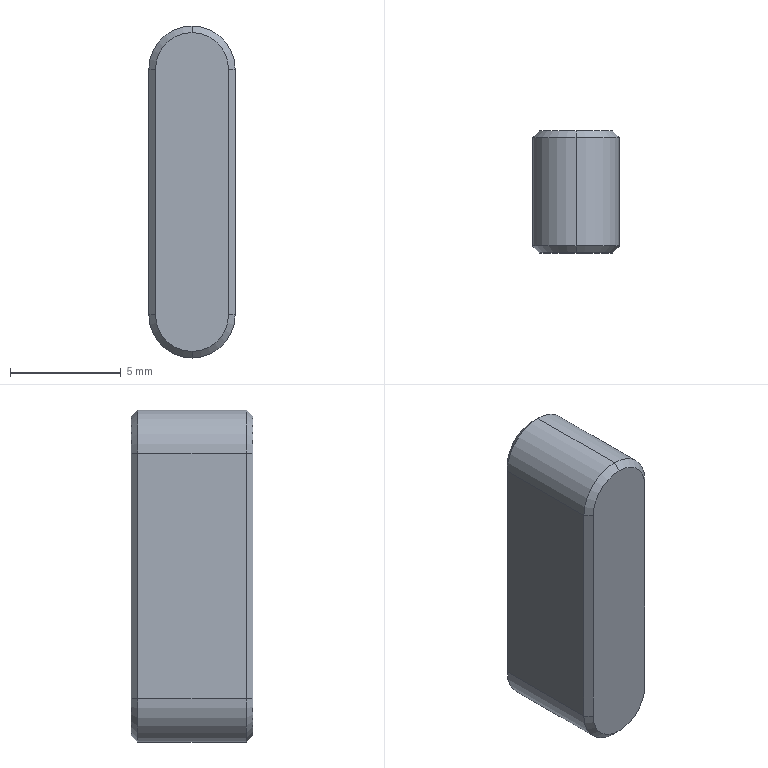Part | STEP file | Key 2 | 1 solid | 20 faces | box 3.9 x 5.5 x 15 mm | volume 300.753 mm3 | plane 8 | cone 8 | cylinder 4 | commonest cylinder face diameters 3.9 x4
STEP:
#1=CARTESIAN_POINT('',(0.,0.,0.));
#2=DIRECTION('',(0.,0.,1.));
#3=DIRECTION('',(1.,0.,0.));
#4=AXIS2_PLACEMENT_3D('',#1,#2,#3);
#5=CARTESIAN_POINT('',(1.95,2.45,13.05));
#6=VERTEX_POINT('',#5);
#7=CARTESIAN_POINT('',(1.95,-2.45,13.05));
#8=VERTEX_POINT('',#7);
#9=CARTESIAN_POINT('',(1.95,-2.75,13.05));
#10=DIRECTION('',(0.,-1.,0.));
#11=VECTOR('',#10,1.);
#12=LINE('',#9,#11);
#13=CARTESIAN_POINT('',(1.95,2.75,15.));
#14=DIRECTION('',(-1.,0.,0.));
#15=DIRECTION('',(0.,-1.,0.));
#16=AXIS2_PLACEMENT_3D('',#13,#14,#15);
#17=PLANE('',#16);
#18=CARTESIAN_POINT('',(5.5,-1.95));
#19=DIRECTION('',(1.,0.));
#20=VECTOR('',#19,1.);
#21=LINE('',#18,#20);
#22=(GEOMETRIC_REPRESENTATION_CONTEXT(2)PARAMETRIC_REPRESENTATION_CONTEXT()REPRESENTATION_CONTEXT('',''));
#23=DEFINITIONAL_REPRESENTATION('',(#21),#22);
#24=PCURVE('',#17,#23);
#25=CARTESIAN_POINT('',(0.,0.,13.05));
#26=DIRECTION('',(0.,-1.,0.));
#27=DIRECTION('',(1.,0.,0.));
#28=AXIS2_PLACEMENT_3D('',#25,#26,#27);
#29=CYLINDRICAL_SURFACE('',#28,1.95);
#30=CARTESIAN_POINT('',(0.,2.75));
#31=DIRECTION('',(0.,1.));
#32=VECTOR('',#31,1.);
#33=LINE('',#30,#32);
#34=(GEOMETRIC_REPRESENTATION_CONTEXT(2)PARAMETRIC_REPRESENTATION_CONTEXT()REPRESENTATION_CONTEXT('',''));
#35=DEFINITIONAL_REPRESENTATION('',(#33),#34);
#36=PCURVE('',#29,#35);
#37=SURFACE_CURVE('',#12,(#24,#36),.PCURVE_S1.);
#38=EDGE_CURVE('',#6,#8,#37,.T.);
#39=ORIENTED_EDGE('',*,*,#38,.T.);
#40=CARTESIAN_POINT('',(1.95,-2.45,1.95));
#41=VERTEX_POINT('',#40);
#42=CARTESIAN_POINT('',(1.95,-2.45,15.));
#43=DIRECTION('',(0.,0.,-1.));
#44=VECTOR('',#43,1.);
#45=LINE('',#42,#44);
#46=CARTESIAN_POINT('',(5.2,0.));
#47=DIRECTION('',(0.,-1.));
#48=VECTOR('',#47,1.);
#49=LINE('',#46,#48);
#50=(GEOMETRIC_REPRESENTATION_CONTEXT(2)PARAMETRIC_REPRESENTATION_CONTEXT()REPRESENTATION_CONTEXT('',''));
#51=DEFINITIONAL_REPRESENTATION('',(#49),#50);
#52=PCURVE('',#17,#51);
#53=CARTESIAN_POINT('',(1.95,-2.45,15.));
#54=DIRECTION('',(-0.7071,0.7071,0.));
#55=DIRECTION('',(0.,0.,-1.));
#56=AXIS2_PLACEMENT_3D('',#53,#54,#55);
#57=PLANE('',#56);
#58=CARTESIAN_POINT('',(0.,0.));
#59=DIRECTION('',(1.,0.));
#60=VECTOR('',#59,1.);
#61=LINE('',#58,#60);
#62=(GEOMETRIC_REPRESENTATION_CONTEXT(2)PARAMETRIC_REPRESENTATION_CONTEXT()REPRESENTATION_CONTEXT('',''));
#63=DEFINITIONAL_REPRESENTATION('',(#61),#62);
#64=PCURVE('',#57,#63);
#65=SURFACE_CURVE('',#45,(#52,#64),.PCURVE_S1.);
#66=EDGE_CURVE('',#8,#41,#65,.T.);
#67=ORIENTED_EDGE('',*,*,#66,.T.);
#68=CARTESIAN_POINT('',(1.95,2.45,1.95));
#69=VERTEX_POINT('',#68);
#70=CARTESIAN_POINT('',(1.95,2.75,1.95));
#71=DIRECTION('',(0.,1.,0.));
#72=VECTOR('',#71,1.);
#73=LINE('',#70,#72);
#74=CARTESIAN_POINT('',(0.,-13.05));
#75=DIRECTION('',(-1.,0.));
#76=VECTOR('',#75,1.);
#77=LINE('',#74,#76);
#78=(GEOMETRIC_REPRESENTATION_CONTEXT(2)PARAMETRIC_REPRESENTATION_CONTEXT()REPRESENTATION_CONTEXT('',''));
#79=DEFINITIONAL_REPRESENTATION('',(#77),#78);
#80=PCURVE('',#17,#79);
#81=CARTESIAN_POINT('',(0.,2.75,1.95));
#82=DIRECTION('',(0.,1.,0.));
#83=DIRECTION('',(-1.,0.,0.));
#84=AXIS2_PLACEMENT_3D('',#81,#82,#83);
#85=CYLINDRICAL_SURFACE('',#84,1.95);
#86=CARTESIAN_POINT('',(3.142,0.));
#87=DIRECTION('',(0.,1.));
#88=VECTOR('',#87,1.);
#89=LINE('',#86,#88);
#90=(GEOMETRIC_REPRESENTATION_CONTEXT(2)PARAMETRIC_REPRESENTATION_CONTEXT()REPRESENTATION_CONTEXT('',''));
#91=DEFINITIONAL_REPRESENTATION('',(#89),#90);
#92=PCURVE('',#85,#91);
#93=SURFACE_CURVE('',#73,(#80,#92),.PCURVE_S1.);
#94=EDGE_CURVE('',#41,#69,#93,.T.);
#95=ORIENTED_EDGE('',*,*,#94,.T.);
#96=CARTESIAN_POINT('',(1.95,2.45,15.));
#97=DIRECTION('',(0.,0.,1.));
#98=VECTOR('',#97,1.);
#99=LINE('',#96,#98);
#100=CARTESIAN_POINT('',(0.3,0.));
#101=DIRECTION('',(0.,1.));
#102=VECTOR('',#101,1.);
#103=LINE('',#100,#102);
#104=(GEOMETRIC_REPRESENTATION_CONTEXT(2)PARAMETRIC_REPRESENTATION_CONTEXT()REPRESENTATION_CONTEXT('',''));
#105=DEFINITIONAL_REPRESENTATION('',(#103),#104);
#106=PCURVE('',#17,#105);
#107=CARTESIAN_POINT('',(1.65,2.75,15.));
#108=DIRECTION('',(-0.7071,-0.7071,0.));
#109=DIRECTION('',(0.,0.,-1.));
#110=AXIS2_PLACEMENT_3D('',#107,#108,#109);
#111=PLANE('',#110);
#112=CARTESIAN_POINT('',(0.,0.4243));
#113=DIRECTION('',(-1.,0.));
#114=VECTOR('',#113,1.);
#115=LINE('',#112,#114);
#116=(GEOMETRIC_REPRESENTATION_CONTEXT(2)PARAMETRIC_REPRESENTATION_CONTEXT()REPRESENTATION_CONTEXT('',''));
#117=DEFINITIONAL_REPRESENTATION('',(#115),#116);
#118=PCURVE('',#111,#117);
#119=SURFACE_CURVE('',#99,(#106,#118),.PCURVE_S1.);
#120=EDGE_CURVE('',#69,#6,#119,.T.);
#121=ORIENTED_EDGE('',*,*,#120,.T.);
#122=EDGE_LOOP('',(#39,#67,#95,#121));
#123=FACE_BOUND('',#122,.T.);
#124=ADVANCED_FACE('',(#123),#17,.F.);
#125=CARTESIAN_POINT('',(0.,2.75,0.3));
#126=VERTEX_POINT('',#125);
#127=CARTESIAN_POINT('',(-1.65,2.75,1.95));
#128=VERTEX_POINT('',#127);
#129=CARTESIAN_POINT('',(0.,2.75,1.95));
#130=DIRECTION('',(0.,1.,0.));
#131=DIRECTION('',(0.,0.,-1.));
#132=AXIS2_PLACEMENT_3D('',#129,#130,#131);
#133=CIRCLE('',#132,1.65);
#134=CARTESIAN_POINT('',(-1.95,2.75,15.));
#135=DIRECTION('',(0.,-1.,0.));
#136=DIRECTION('',(0.,0.,-1.));
#137=AXIS2_PLACEMENT_3D('',#134,#135,#136);
#138=PLANE('',#137);
#139=CARTESIAN_POINT('',(14.7,1.95));
#140=CARTESIAN_POINT('',(14.7,-0.9079));
#141=CARTESIAN_POINT('',(12.225,0.5211));
#142=CARTESIAN_POINT('',(9.75,1.95));
#143=CARTESIAN_POINT('',(12.225,3.379));
#144=CARTESIAN_POINT('',(14.7,4.808));
#145=CARTESIAN_POINT('',(14.7,1.95));
#146=(BOUNDED_CURVE()B_SPLINE_CURVE(2,(#139,#140,#141,#142,#143,#144,#145),.UNSPECIFIED.,.T.,.F.)B_SPLINE_CURVE_WITH_KNOTS((1,2,2,2,2,1),(-2.094,0.,2.094,4.189,6.283,8.378),.UNSPECIFIED.)CURVE()GEOMETRIC_REPRESENTATION_ITEM()RATIONAL_B_SPLINE_CURVE((1.,0.5,1.,0.5,1.,0.5,1.))REPRESENTATION_ITEM(''));
#147=(GEOMETRIC_REPRESENTATION_CONTEXT(2)PARAMETRIC_REPRESENTATION_CONTEXT()REPRESENTATION_CONTEXT('',''));
#148=DEFINITIONAL_REPRESENTATION('',(#146),#147);
#149=PCURVE('',#138,#148);
#150=CARTESIAN_POINT('',(0.,2.75,1.95));
#151=DIRECTION('',(0.,-1.,0.));
#152=DIRECTION('',(1.,0.,0.));
#153=AXIS2_PLACEMENT_3D('',#150,#151,#152);
#154=CONICAL_SURFACE('',#153,1.65,0.7854);
#155=CARTESIAN_POINT('',(4.712,0.));
#156=DIRECTION('',(-1.,0.));
#157=VECTOR('',#156,1.);
#158=LINE('',#155,#157);
#159=(GEOMETRIC_REPRESENTATION_CONTEXT(2)PARAMETRIC_REPRESENTATION_CONTEXT()REPRESENTATION_CONTEXT('',''));
#160=DEFINITIONAL_REPRESENTATION('',(#158),#159);
#161=PCURVE('',#154,#160);
#162=SURFACE_CURVE('',#133,(#149,#161),.PCURVE_S1.);
#163=EDGE_CURVE('',#126,#128,#162,.T.);
#164=ORIENTED_EDGE('',*,*,#163,.T.);
#165=CARTESIAN_POINT('',(-1.65,2.75,13.05));
#166=VERTEX_POINT('',#165);
#167=CARTESIAN_POINT('',(-1.65,2.75,15.));
#168=DIRECTION('',(0.,0.,1.));
#169=VECTOR('',#168,1.);
#170=LINE('',#167,#169);
#171=CARTESIAN_POINT('',(0.,0.3));
#172=DIRECTION('',(-1.,0.));
#173=VECTOR('',#172,1.);
#174=LINE('',#171,#173);
#175=(GEOMETRIC_REPRESENTATION_CONTEXT(2)PARAMETRIC_REPRESENTATION_CONTEXT()REPRESENTATION_CONTEXT('',''));
#176=DEFINITIONAL_REPRESENTATION('',(#174),#175);
#177=PCURVE('',#138,#176);
#178=CARTESIAN_POINT('',(-1.95,2.45,15.));
#179=DIRECTION('',(0.7071,-0.7071,0.));
#180=DIRECTION('',(0.,0.,-1.));
#181=AXIS2_PLACEMENT_3D('',#178,#179,#180);
#182=PLANE('',#181);
#183=CARTESIAN_POINT('',(0.,0.4243));
#184=DIRECTION('',(-1.,0.));
#185=VECTOR('',#184,1.);
#186=LINE('',#183,#185);
#187=(GEOMETRIC_REPRESENTATION_CONTEXT(2)PARAMETRIC_REPRESENTATION_CONTEXT()REPRESENTATION_CONTEXT('',''));
#188=DEFINITIONAL_REPRESENTATION('',(#186),#187);
#189=PCURVE('',#182,#188);
#190=SURFACE_CURVE('',#170,(#177,#189),.PCURVE_S1.);
#191=EDGE_CURVE('',#128,#166,#190,.T.);
#192=ORIENTED_EDGE('',*,*,#191,.T.);
#193=CARTESIAN_POINT('',(0.,2.75,14.7));
#194=VERTEX_POINT('',#193);
#195=CARTESIAN_POINT('',(0.,2.75,13.05));
#196=DIRECTION('',(0.,1.,0.));
#197=DIRECTION('',(0.,0.,-1.));
#198=AXIS2_PLACEMENT_3D('',#195,#196,#197);
#199=CIRCLE('',#198,1.65);
#200=CARTESIAN_POINT('',(3.6,1.95));
#201=CARTESIAN_POINT('',(3.6,-0.9079));
#202=CARTESIAN_POINT('',(1.125,0.5211));
#203=CARTESIAN_POINT('',(-1.35,1.95));
#204=CARTESIAN_POINT('',(1.125,3.379));
#205=CARTESIAN_POINT('',(3.6,4.808));
#206=CARTESIAN_POINT('',(3.6,1.95));
#207=(BOUNDED_CURVE()B_SPLINE_CURVE(2,(#200,#201,#202,#203,#204,#205,#206),.UNSPECIFIED.,.T.,.F.)B_SPLINE_CURVE_WITH_KNOTS((1,2,2,2,2,1),(-2.094,0.,2.094,4.189,6.283,8.378),.UNSPECIFIED.)CURVE()GEOMETRIC_REPRESENTATION_ITEM()RATIONAL_B_SPLINE_CURVE((1.,0.5,1.,0.5,1.,0.5,1.))REPRESENTATION_ITEM(''));
#208=(GEOMETRIC_REPRESENTATION_CONTEXT(2)PARAMETRIC_REPRESENTATION_CONTEXT()REPRESENTATION_CONTEXT('',''));
#209=DEFINITIONAL_REPRESENTATION('',(#207),#208);
#210=PCURVE('',#138,#209);
#211=CARTESIAN_POINT('',(0.,2.75,13.05));
#212=DIRECTION('',(0.,-1.,0.));
#213=DIRECTION('',(1.,0.,0.));
#214=AXIS2_PLACEMENT_3D('',#211,#212,#213);
#215=CONICAL_SURFACE('',#214,1.65,0.7854);
#216=CARTESIAN_POINT('',(4.712,0.));
#217=DIRECTION('',(-1.,0.));
#218=VECTOR('',#217,1.);
#219=LINE('',#216,#218);
#220=(GEOMETRIC_REPRESENTATION_CONTEXT(2)PARAMETRIC_REPRESENTATION_CONTEXT()REPRESENTATION_CONTEXT('',''));
#221=DEFINITIONAL_REPRESENTATION('',(#219),#220);
#222=PCURVE('',#215,#221);
#223=SURFACE_CURVE('',#199,(#210,#222),.PCURVE_S1.);
#224=EDGE_CURVE('',#166,#194,#223,.T.);
#225=ORIENTED_EDGE('',*,*,#224,.T.);
#226=CARTESIAN_POINT('',(1.65,2.75,13.05));
#227=VERTEX_POINT('',#226);
#228=CARTESIAN_POINT('',(0.,2.75,13.05));
#229=DIRECTION('',(0.,1.,0.));
#230=DIRECTION('',(0.,0.,-1.));
#231=AXIS2_PLACEMENT_3D('',#228,#229,#230);
#232=CIRCLE('',#231,1.65);
#233=CARTESIAN_POINT('',(3.6,1.95));
#234=CARTESIAN_POINT('',(3.6,-0.9079));
#235=CARTESIAN_POINT('',(1.125,0.5211));
#236=CARTESIAN_POINT('',(-1.35,1.95));
#237=CARTESIAN_POINT('',(1.125,3.379));
#238=CARTESIAN_POINT('',(3.6,4.808));
#239=CARTESIAN_POINT('',(3.6,1.95));
#240=(BOUNDED_CURVE()B_SPLINE_CURVE(2,(#233,#234,#235,#236,#237,#238,#239),.UNSPECIFIED.,.T.,.F.)B_SPLINE_CURVE_WITH_KNOTS((1,2,2,2,2,1),(-2.094,0.,2.094,4.189,6.283,8.378),.UNSPECIFIED.)CURVE()GEOMETRIC_REPRESENTATION_ITEM()RATIONAL_B_SPLINE_CURVE((1.,0.5,1.,0.5,1.,0.5,1.))REPRESENTATION_ITEM(''));
#241=(GEOMETRIC_REPRESENTATION_CONTEXT(2)PARAMETRIC_REPRESENTATION_CONTEXT()REPRESENTATION_CONTEXT('',''));
#242=DEFINITIONAL_REPRESENTATION('',(#240),#241);
#243=PCURVE('',#138,#242);
#244=CARTESIAN_POINT('',(0.,2.75,13.05));
#245=DIRECTION('',(0.,-1.,0.));
#246=DIRECTION('',(1.,0.,0.));
#247=AXIS2_PLACEMENT_3D('',#244,#245,#246);
#248=CONICAL_SURFACE('',#247,1.65,0.7854);
#249=CARTESIAN_POINT('',(4.712,0.));
#250=DIRECTION('',(-1.,0.));
#251=VECTOR('',#250,1.);
#252=LINE('',#249,#251);
#253=(GEOMETRIC_REPRESENTATION_CONTEXT(2)PARAMETRIC_REPRESENTATION_CONTEXT()REPRESENTATION_CONTEXT('',''));
#254=DEFINITIONAL_REPRESENTATION('',(#252),#253);
#255=PCURVE('',#248,#254);
#256=SURFACE_CURVE('',#232,(#243,#255),.PCURVE_S1.);
#257=EDGE_CURVE('',#194,#227,#256,.T.);
#258=ORIENTED_EDGE('',*,*,#257,.T.);
#259=CARTESIAN_POINT('',(1.65,2.75,1.95));
#260=VERTEX_POINT('',#259);
#261=CARTESIAN_POINT('',(1.65,2.75,15.));
#262=DIRECTION('',(0.,0.,-1.));
#263=VECTOR('',#262,1.);
#264=LINE('',#261,#263);
#265=CARTESIAN_POINT('',(0.,3.6));
#266=DIRECTION('',(1.,0.));
#267=VECTOR('',#266,1.);
#268=LINE('',#265,#267);
#269=(GEOMETRIC_REPRESENTATION_CONTEXT(2)PARAMETRIC_REPRESENTATION_CONTEXT()REPRESENTATION_CONTEXT('',''));
#270=DEFINITIONAL_REPRESENTATION('',(#268),#269);
#271=PCURVE('',#138,#270);
#272=CARTESIAN_POINT('',(0.,0.));
#273=DIRECTION('',(1.,0.));
#274=VECTOR('',#273,1.);
#275=LINE('',#272,#274);
#276=(GEOMETRIC_REPRESENTATION_CONTEXT(2)PARAMETRIC_REPRESENTATION_CONTEXT()REPRESENTATION_CONTEXT('',''));
#277=DEFINITIONAL_REPRESENTATION('',(#275),#276);
#278=PCURVE('',#111,#277);
#279=SURFACE_CURVE('',#264,(#271,#278),.PCURVE_S1.);
#280=EDGE_CURVE('',#227,#260,#279,.T.);
#281=ORIENTED_EDGE('',*,*,#280,.T.);
#282=CARTESIAN_POINT('',(0.,2.75,1.95));
#283=DIRECTION('',(0.,1.,0.));
#284=DIRECTION('',(0.,0.,-1.));
#285=AXIS2_PLACEMENT_3D('',#282,#283,#284);
#286=CIRCLE('',#285,1.65);
#287=CARTESIAN_POINT('',(14.7,1.95));
#288=CARTESIAN_POINT('',(14.7,-0.9079));
#289=CARTESIAN_POINT('',(12.225,0.5211));
#290=CARTESIAN_POINT('',(9.75,1.95));
#291=CARTESIAN_POINT('',(12.225,3.379));
#292=CARTESIAN_POINT('',(14.7,4.808));
#293=CARTESIAN_POINT('',(14.7,1.95));
#294=(BOUNDED_CURVE()B_SPLINE_CURVE(2,(#287,#288,#289,#290,#291,#292,#293),.UNSPECIFIED.,.T.,.F.)B_SPLINE_CURVE_WITH_KNOTS((1,2,2,2,2,1),(-2.094,0.,2.094,4.189,6.283,8.378),.UNSPECIFIED.)CURVE()GEOMETRIC_REPRESENTATION_ITEM()RATIONAL_B_SPLINE_CURVE((1.,0.5,1.,0.5,1.,0.5,1.))REPRESENTATION_ITEM(''));
#295=(GEOMETRIC_REPRESENTATION_CONTEXT(2)PARAMETRIC_REPRESENTATION_CONTEXT()REPRESENTATION_CONTEXT('',''));
#296=DEFINITIONAL_REPRESENTATION('',(#294),#295);
#297=PCURVE('',#138,#296);
#298=CARTESIAN_POINT('',(0.,2.75,1.95));
#299=DIRECTION('',(0.,-1.,0.));
#300=DIRECTION('',(1.,0.,0.));
#301=AXIS2_PLACEMENT_3D('',#298,#299,#300);
#302=CONICAL_SURFACE('',#301,1.65,0.7854);
#303=CARTESIAN_POINT('',(10.996,0.));
#304=DIRECTION('',(-1.,0.));
#305=VECTOR('',#304,1.);
#306=LINE('',#303,#305);
#307=(GEOMETRIC_REPRESENTATION_CONTEXT(2)PARAMETRIC_REPRESENTATION_CONTEXT()REPRESENTATION_CONTEXT('',''));
#308=DEFINITIONAL_REPRESENTATION('',(#306),#307);
#309=PCURVE('',#302,#308);
#310=SURFACE_CURVE('',#286,(#297,#309),.PCURVE_S1.);
#311=EDGE_CURVE('',#260,#126,#310,.T.);
#312=ORIENTED_EDGE('',*,*,#311,.T.);
#313=EDGE_LOOP('',(#164,#192,#225,#258,#281,#312));
#314=FACE_BOUND('',#313,.T.);
#315=ADVANCED_FACE('',(#314),#138,.F.);
#316=CARTESIAN_POINT('',(-1.95,2.45,1.95));
#317=VERTEX_POINT('',#316);
#318=CARTESIAN_POINT('',(-1.95,-2.45,1.95));
#319=VERTEX_POINT('',#318);
#320=CARTESIAN_POINT('',(-1.95,2.75,1.95));
#321=DIRECTION('',(0.,-1.,0.));
#322=VECTOR('',#321,1.);
#323=LINE('',#320,#322);
#324=CARTESIAN_POINT('',(-1.95,2.75,15.));
#325=DIRECTION('',(1.,0.,0.));
#326=DIRECTION('',(0.,1.,0.));
#327=AXIS2_PLACEMENT_3D('',#324,#325,#326);
#328=PLANE('',#327);
#329=CARTESIAN_POINT('',(0.,-13.05));
#330=DIRECTION('',(-1.,0.));
#331=VECTOR('',#330,1.);
#332=LINE('',#329,#331);
#333=(GEOMETRIC_REPRESENTATION_CONTEXT(2)PARAMETRIC_REPRESENTATION_CONTEXT()REPRESENTATION_CONTEXT('',''));
#334=DEFINITIONAL_REPRESENTATION('',(#332),#333);
#335=PCURVE('',#328,#334);
#336=CARTESIAN_POINT('',(0.,2.75,1.95));
#337=DIRECTION('',(0.,-1.,0.));
#338=DIRECTION('',(1.,0.,0.));
#339=AXIS2_PLACEMENT_3D('',#336,#337,#338);
#340=CYLINDRICAL_SURFACE('',#339,1.95);
#341=CARTESIAN_POINT('',(3.142,0.));
#342=DIRECTION('',(0.,1.));
#343=VECTOR('',#342,1.);
#344=LINE('',#341,#343);
#345=(GEOMETRIC_REPRESENTATION_CONTEXT(2)PARAMETRIC_REPRESENTATION_CONTEXT()REPRESENTATION_CONTEXT('',''));
#346=DEFINITIONAL_REPRESENTATION('',(#344),#345);
#347=PCURVE('',#340,#346);
#348=SURFACE_CURVE('',#323,(#335,#347),.PCURVE_S1.);
#349=EDGE_CURVE('',#317,#319,#348,.T.);
#350=ORIENTED_EDGE('',*,*,#349,.T.);
#351=CARTESIAN_POINT('',(-1.95,-2.45,13.05));
#352=VERTEX_POINT('',#351);
#353=CARTESIAN_POINT('',(-1.95,-2.45,15.));
#354=DIRECTION('',(0.,0.,1.));
#355=VECTOR('',#354,1.);
#356=LINE('',#353,#355);
#357=CARTESIAN_POINT('',(-5.2,0.));
#358=DIRECTION('',(0.,1.));
#359=VECTOR('',#358,1.);
#360=LINE('',#357,#359);
#361=(GEOMETRIC_REPRESENTATION_CONTEXT(2)PARAMETRIC_REPRESENTATION_CONTEXT()REPRESENTATION_CONTEXT('',''));
#362=DEFINITIONAL_REPRESENTATION('',(#360),#361);
#363=PCURVE('',#328,#362);
#364=CARTESIAN_POINT('',(-1.65,-2.75,15.));
#365=DIRECTION('',(0.7071,0.7071,0.));
#366=DIRECTION('',(0.,0.,-1.));
#367=AXIS2_PLACEMENT_3D('',#364,#365,#366);
#368=PLANE('',#367);
#369=CARTESIAN_POINT('',(0.,0.4243));
#370=DIRECTION('',(-1.,0.));
#371=VECTOR('',#370,1.);
#372=LINE('',#369,#371);
#373=(GEOMETRIC_REPRESENTATION_CONTEXT(2)PARAMETRIC_REPRESENTATION_CONTEXT()REPRESENTATION_CONTEXT('',''));
#374=DEFINITIONAL_REPRESENTATION('',(#372),#373);
#375=PCURVE('',#368,#374);
#376=SURFACE_CURVE('',#356,(#363,#375),.PCURVE_S1.);
#377=EDGE_CURVE('',#319,#352,#376,.T.);
#378=ORIENTED_EDGE('',*,*,#377,.T.);
#379=CARTESIAN_POINT('',(-1.95,2.45,13.05));
#380=VERTEX_POINT('',#379);
#381=CARTESIAN_POINT('',(-1.95,2.75,13.05));
#382=DIRECTION('',(0.,1.,0.));
#383=VECTOR('',#382,1.);
#384=LINE('',#381,#383);
#385=CARTESIAN_POINT('',(0.,-1.95));
#386=DIRECTION('',(1.,0.));
#387=VECTOR('',#386,1.);
#388=LINE('',#385,#387);
#389=(GEOMETRIC_REPRESENTATION_CONTEXT(2)PARAMETRIC_REPRESENTATION_CONTEXT()REPRESENTATION_CONTEXT('',''));
#390=DEFINITIONAL_REPRESENTATION('',(#388),#389);
#391=PCURVE('',#328,#390);
#392=CARTESIAN_POINT('',(0.,0.,13.05));
#393=DIRECTION('',(0.,1.,0.));
#394=DIRECTION('',(-1.,0.,0.));
#395=AXIS2_PLACEMENT_3D('',#392,#393,#394);
#396=CYLINDRICAL_SURFACE('',#395,1.95);
#397=CARTESIAN_POINT('',(0.,2.75));
#398=DIRECTION('',(0.,1.));
#399=VECTOR('',#398,1.);
#400=LINE('',#397,#399);
#401=(GEOMETRIC_REPRESENTATION_CONTEXT(2)PARAMETRIC_REPRESENTATION_CONTEXT()REPRESENTATION_CONTEXT('',''));
#402=DEFINITIONAL_REPRESENTATION('',(#400),#401);
#403=PCURVE('',#396,#402);
#404=SURFACE_CURVE('',#384,(#391,#403),.PCURVE_S1.);
#405=EDGE_CURVE('',#352,#380,#404,.T.);
#406=ORIENTED_EDGE('',*,*,#405,.T.);
#407=CARTESIAN_POINT('',(-1.95,2.45,15.));
#408=DIRECTION('',(0.,0.,-1.));
#409=VECTOR('',#408,1.);
#410=LINE('',#407,#409);
#411=CARTESIAN_POINT('',(-0.3,0.));
#412=DIRECTION('',(0.,-1.));
#413=VECTOR('',#412,1.);
#414=LINE('',#411,#413);
#415=(GEOMETRIC_REPRESENTATION_CONTEXT(2)PARAMETRIC_REPRESENTATION_CONTEXT()REPRESENTATION_CONTEXT('',''));
#416=DEFINITIONAL_REPRESENTATION('',(#414),#415);
#417=PCURVE('',#328,#416);
#418=CARTESIAN_POINT('',(0.,0.));
#419=DIRECTION('',(1.,0.));
#420=VECTOR('',#419,1.);
#421=LINE('',#418,#420);
#422=(GEOMETRIC_REPRESENTATION_CONTEXT(2)PARAMETRIC_REPRESENTATION_CONTEXT()REPRESENTATION_CONTEXT('',''));
#423=DEFINITIONAL_REPRESENTATION('',(#421),#422);
#424=PCURVE('',#182,#423);
#425=SURFACE_CURVE('',#410,(#417,#424),.PCURVE_S1.);
#426=EDGE_CURVE('',#380,#317,#425,.T.);
#427=ORIENTED_EDGE('',*,*,#426,.T.);
#428=EDGE_LOOP('',(#350,#378,#406,#427));
#429=FACE_BOUND('',#428,.T.);
#430=ADVANCED_FACE('',(#429),#328,.F.);
#431=CARTESIAN_POINT('',(0.,-2.75,14.7));
#432=VERTEX_POINT('',#431);
#433=CARTESIAN_POINT('',(-1.65,-2.75,13.05));
#434=VERTEX_POINT('',#433);
#435=CARTESIAN_POINT('',(0.,-2.75,13.05));
#436=DIRECTION('',(0.,-1.,0.));
#437=DIRECTION('',(0.,0.,1.));
#438=AXIS2_PLACEMENT_3D('',#435,#436,#437);
#439=CIRCLE('',#438,1.65);
#440=CARTESIAN_POINT('',(-1.95,-2.75,15.));
#441=DIRECTION('',(0.,1.,0.));
#442=DIRECTION('',(0.,0.,1.));
#443=AXIS2_PLACEMENT_3D('',#440,#441,#442);
#444=PLANE('',#443);
#445=CARTESIAN_POINT('',(-0.3,1.95));
#446=CARTESIAN_POINT('',(-0.3,-0.9079));
#447=CARTESIAN_POINT('',(-2.775,0.5211));
#448=CARTESIAN_POINT('',(-5.25,1.95));
#449=CARTESIAN_POINT('',(-2.775,3.379));
#450=CARTESIAN_POINT('',(-0.3,4.808));
#451=CARTESIAN_POINT('',(-0.3,1.95));
#452=(BOUNDED_CURVE()B_SPLINE_CURVE(2,(#445,#446,#447,#448,#449,#450,#451),.UNSPECIFIED.,.T.,.F.)B_SPLINE_CURVE_WITH_KNOTS((1,2,2,2,2,1),(-2.094,0.,2.094,4.189,6.283,8.378),.UNSPECIFIED.)CURVE()GEOMETRIC_REPRESENTATION_ITEM()RATIONAL_B_SPLINE_CURVE((1.,0.5,1.,0.5,1.,0.5,1.))REPRESENTATION_ITEM(''));
#453=(GEOMETRIC_REPRESENTATION_CONTEXT(2)PARAMETRIC_REPRESENTATION_CONTEXT()REPRESENTATION_CONTEXT('',''));
#454=DEFINITIONAL_REPRESENTATION('',(#452),#453);
#455=PCURVE('',#444,#454);
#456=CARTESIAN_POINT('',(0.,-2.75,13.05));
#457=DIRECTION('',(0.,1.,0.));
#458=DIRECTION('',(-1.,0.,0.));
#459=AXIS2_PLACEMENT_3D('',#456,#457,#458);
#460=CONICAL_SURFACE('',#459,1.65,0.7854);
#461=CARTESIAN_POINT('',(1.571,0.));
#462=DIRECTION('',(-1.,0.));
#463=VECTOR('',#462,1.);
#464=LINE('',#461,#463);
#465=(GEOMETRIC_REPRESENTATION_CONTEXT(2)PARAMETRIC_REPRESENTATION_CONTEXT()REPRESENTATION_CONTEXT('',''));
#466=DEFINITIONAL_REPRESENTATION('',(#464),#465);
#467=PCURVE('',#460,#466);
#468=SURFACE_CURVE('',#439,(#455,#467),.PCURVE_S1.);
#469=EDGE_CURVE('',#432,#434,#468,.T.);
#470=ORIENTED_EDGE('',*,*,#469,.T.);
#471=CARTESIAN_POINT('',(-1.65,-2.75,1.95));
#472=VERTEX_POINT('',#471);
#473=CARTESIAN_POINT('',(-1.65,-2.75,15.));
#474=DIRECTION('',(0.,0.,-1.));
#475=VECTOR('',#474,1.);
#476=LINE('',#473,#475);
#477=CARTESIAN_POINT('',(0.,0.3));
#478=DIRECTION('',(-1.,0.));
#479=VECTOR('',#478,1.);
#480=LINE('',#477,#479);
#481=(GEOMETRIC_REPRESENTATION_CONTEXT(2)PARAMETRIC_REPRESENTATION_CONTEXT()REPRESENTATION_CONTEXT('',''));
#482=DEFINITIONAL_REPRESENTATION('',(#480),#481);
#483=PCURVE('',#444,#482);
#484=CARTESIAN_POINT('',(0.,0.));
#485=DIRECTION('',(1.,0.));
#486=VECTOR('',#485,1.);
#487=LINE('',#484,#486);
#488=(GEOMETRIC_REPRESENTATION_CONTEXT(2)PARAMETRIC_REPRESENTATION_CONTEXT()REPRESENTATION_CONTEXT('',''));
#489=DEFINITIONAL_REPRESENTATION('',(#487),#488);
#490=PCURVE('',#368,#489);
#491=SURFACE_CURVE('',#476,(#483,#490),.PCURVE_S1.);
#492=EDGE_CURVE('',#434,#472,#491,.T.);
#493=ORIENTED_EDGE('',*,*,#492,.T.);
#494=CARTESIAN_POINT('',(0.,-2.75,0.3));
#495=VERTEX_POINT('',#494);
#496=CARTESIAN_POINT('',(0.,-2.75,1.95));
#497=DIRECTION('',(0.,-1.,0.));
#498=DIRECTION('',(0.,0.,1.));
#499=AXIS2_PLACEMENT_3D('',#496,#497,#498);
#500=CIRCLE('',#499,1.65);
#501=CARTESIAN_POINT('',(-11.4,1.95));
#502=CARTESIAN_POINT('',(-11.4,-0.9079));
#503=CARTESIAN_POINT('',(-13.875,0.5211));
#504=CARTESIAN_POINT('',(-16.35,1.95));
#505=CARTESIAN_POINT('',(-13.875,3.379));
#506=CARTESIAN_POINT('',(-11.4,4.808));
#507=CARTESIAN_POINT('',(-11.4,1.95));
#508=(BOUNDED_CURVE()B_SPLINE_CURVE(2,(#501,#502,#503,#504,#505,#506,#507),.UNSPECIFIED.,.T.,.F.)B_SPLINE_CURVE_WITH_KNOTS((1,2,2,2,2,1),(-2.094,0.,2.094,4.189,6.283,8.378),.UNSPECIFIED.)CURVE()GEOMETRIC_REPRESENTATION_ITEM()RATIONAL_B_SPLINE_CURVE((1.,0.5,1.,0.5,1.,0.5,1.))REPRESENTATION_ITEM(''));
#509=(GEOMETRIC_REPRESENTATION_CONTEXT(2)PARAMETRIC_REPRESENTATION_CONTEXT()REPRESENTATION_CONTEXT('',''));
#510=DEFINITIONAL_REPRESENTATION('',(#508),#509);
#511=PCURVE('',#444,#510);
#512=CARTESIAN_POINT('',(0.,-2.75,1.95));
#513=DIRECTION('',(0.,1.,0.));
#514=DIRECTION('',(-1.,0.,0.));
#515=AXIS2_PLACEMENT_3D('',#512,#513,#514);
#516=CONICAL_SURFACE('',#515,1.65,0.7854);
#517=CARTESIAN_POINT('',(7.854,0.));
#518=DIRECTION('',(-1.,0.));
#519=VECTOR('',#518,1.);
#520=LINE('',#517,#519);
#521=(GEOMETRIC_REPRESENTATION_CONTEXT(2)PARAMETRIC_REPRESENTATION_CONTEXT()REPRESENTATION_CONTEXT('',''));
#522=DEFINITIONAL_REPRESENTATION('',(#520),#521);
#523=PCURVE('',#516,#522);
#524=SURFACE_CURVE('',#500,(#511,#523),.PCURVE_S1.);
#525=EDGE_CURVE('',#472,#495,#524,.T.);
#526=ORIENTED_EDGE('',*,*,#525,.T.);
#527=CARTESIAN_POINT('',(1.65,-2.75,1.95));
#528=VERTEX_POINT('',#527);
#529=CARTESIAN_POINT('',(0.,-2.75,1.95));
#530=DIRECTION('',(0.,-1.,0.));
#531=DIRECTION('',(0.,0.,1.));
#532=AXIS2_PLACEMENT_3D('',#529,#530,#531);
#533=CIRCLE('',#532,1.65);
#534=CARTESIAN_POINT('',(-11.4,1.95));
#535=CARTESIAN_POINT('',(-11.4,-0.9079));
#536=CARTESIAN_POINT('',(-13.875,0.5211));
#537=CARTESIAN_POINT('',(-16.35,1.95));
#538=CARTESIAN_POINT('',(-13.875,3.379));
#539=CARTESIAN_POINT('',(-11.4,4.808));
#540=CARTESIAN_POINT('',(-11.4,1.95));
#541=(BOUNDED_CURVE()B_SPLINE_CURVE(2,(#534,#535,#536,#537,#538,#539,#540),.UNSPECIFIED.,.T.,.F.)B_SPLINE_CURVE_WITH_KNOTS((1,2,2,2,2,1),(-2.094,0.,2.094,4.189,6.283,8.378),.UNSPECIFIED.)CURVE()GEOMETRIC_REPRESENTATION_ITEM()RATIONAL_B_SPLINE_CURVE((1.,0.5,1.,0.5,1.,0.5,1.))REPRESENTATION_ITEM(''));
#542=(GEOMETRIC_REPRESENTATION_CONTEXT(2)PARAMETRIC_REPRESENTATION_CONTEXT()REPRESENTATION_CONTEXT('',''));
#543=DEFINITIONAL_REPRESENTATION('',(#541),#542);
#544=PCURVE('',#444,#543);
#545=CARTESIAN_POINT('',(0.,-2.75,1.95));
#546=DIRECTION('',(0.,1.,0.));
#547=DIRECTION('',(-1.,0.,0.));
#548=AXIS2_PLACEMENT_3D('',#545,#546,#547);
#549=CONICAL_SURFACE('',#548,1.65,0.7854);
#550=CARTESIAN_POINT('',(7.854,0.));
#551=DIRECTION('',(-1.,0.));
#552=VECTOR('',#551,1.);
#553=LINE('',#550,#552);
#554=(GEOMETRIC_REPRESENTATION_CONTEXT(2)PARAMETRIC_REPRESENTATION_CONTEXT()REPRESENTATION_CONTEXT('',''));
#555=DEFINITIONAL_REPRESENTATION('',(#553),#554);
#556=PCURVE('',#549,#555);
#557=SURFACE_CURVE('',#533,(#544,#556),.PCURVE_S1.);
#558=EDGE_CURVE('',#495,#528,#557,.T.);
#559=ORIENTED_EDGE('',*,*,#558,.T.);
#560=CARTESIAN_POINT('',(1.65,-2.75,13.05));
#561=VERTEX_POINT('',#560);
#562=CARTESIAN_POINT('',(1.65,-2.75,15.));
#563=DIRECTION('',(0.,0.,1.));
#564=VECTOR('',#563,1.);
#565=LINE('',#562,#564);
#566=CARTESIAN_POINT('',(0.,3.6));
#567=DIRECTION('',(1.,0.));
#568=VECTOR('',#567,1.);
#569=LINE('',#566,#568);
#570=(GEOMETRIC_REPRESENTATION_CONTEXT(2)PARAMETRIC_REPRESENTATION_CONTEXT()REPRESENTATION_CONTEXT('',''));
#571=DEFINITIONAL_REPRESENTATION('',(#569),#570);
#572=PCURVE('',#444,#571);
#573=CARTESIAN_POINT('',(0.,0.4243));
#574=DIRECTION('',(-1.,0.));
#575=VECTOR('',#574,1.);
#576=LINE('',#573,#575);
#577=(GEOMETRIC_REPRESENTATION_CONTEXT(2)PARAMETRIC_REPRESENTATION_CONTEXT()REPRESENTATION_CONTEXT('',''));
#578=DEFINITIONAL_REPRESENTATION('',(#576),#577);
#579=PCURVE('',#57,#578);
#580=SURFACE_CURVE('',#565,(#572,#579),.PCURVE_S1.);
#581=EDGE_CURVE('',#528,#561,#580,.T.);
#582=ORIENTED_EDGE('',*,*,#581,.T.);
#583=CARTESIAN_POINT('',(0.,-2.75,13.05));
#584=DIRECTION('',(0.,-1.,0.));
#585=DIRECTION('',(0.,0.,1.));
#586=AXIS2_PLACEMENT_3D('',#583,#584,#585);
#587=CIRCLE('',#586,1.65);
#588=CARTESIAN_POINT('',(-0.3,1.95));
#589=CARTESIAN_POINT('',(-0.3,-0.9079));
#590=CARTESIAN_POINT('',(-2.775,0.5211));
#591=CARTESIAN_POINT('',(-5.25,1.95));
#592=CARTESIAN_POINT('',(-2.775,3.379));
#593=CARTESIAN_POINT('',(-0.3,4.808));
#594=CARTESIAN_POINT('',(-0.3,1.95));
#595=(BOUNDED_CURVE()B_SPLINE_CURVE(2,(#588,#589,#590,#591,#592,#593,#594),.UNSPECIFIED.,.T.,.F.)B_SPLINE_CURVE_WITH_KNOTS((1,2,2,2,2,1),(-2.094,0.,2.094,4.189,6.283,8.378),.UNSPECIFIED.)CURVE()GEOMETRIC_REPRESENTATION_ITEM()RATIONAL_B_SPLINE_CURVE((1.,0.5,1.,0.5,1.,0.5,1.))REPRESENTATION_ITEM(''));
#596=(GEOMETRIC_REPRESENTATION_CONTEXT(2)PARAMETRIC_REPRESENTATION_CONTEXT()REPRESENTATION_CONTEXT('',''));
#597=DEFINITIONAL_REPRESENTATION('',(#595),#596);
#598=PCURVE('',#444,#597);
#599=CARTESIAN_POINT('',(0.,-2.75,13.05));
#600=DIRECTION('',(0.,1.,0.));
#601=DIRECTION('',(-1.,0.,0.));
#602=AXIS2_PLACEMENT_3D('',#599,#600,#601);
#603=CONICAL_SURFACE('',#602,1.65,0.7854);
#604=CARTESIAN_POINT('',(7.854,0.));
#605=DIRECTION('',(-1.,0.));
#606=VECTOR('',#605,1.);
#607=LINE('',#604,#606);
#608=(GEOMETRIC_REPRESENTATION_CONTEXT(2)PARAMETRIC_REPRESENTATION_CONTEXT()REPRESENTATION_CONTEXT('',''));
#609=DEFINITIONAL_REPRESENTATION('',(#607),#608);
#610=PCURVE('',#603,#609);
#611=SURFACE_CURVE('',#587,(#598,#610),.PCURVE_S1.);
#612=EDGE_CURVE('',#561,#432,#611,.T.);
#613=ORIENTED_EDGE('',*,*,#612,.T.);
#614=EDGE_LOOP('',(#470,#493,#526,#559,#582,#613));
#615=FACE_BOUND('',#614,.T.);
#616=ADVANCED_FACE('',(#615),#444,.F.);
#617=ORIENTED_EDGE('',*,*,#94,.F.);
#618=CARTESIAN_POINT('',(0.,-2.45,0.));
#619=VERTEX_POINT('',#618);
#620=CARTESIAN_POINT('',(0.,-2.45,1.95));
#621=DIRECTION('',(0.,1.,0.));
#622=DIRECTION('',(-1.,0.,0.));
#623=AXIS2_PLACEMENT_3D('',#620,#621,#622);
#624=CIRCLE('',#623,1.95);
#625=CARTESIAN_POINT('',(0.,-5.2));
#626=DIRECTION('',(1.,0.));
#627=VECTOR('',#626,1.);
#628=LINE('',#625,#627);
#629=(GEOMETRIC_REPRESENTATION_CONTEXT(2)PARAMETRIC_REPRESENTATION_CONTEXT()REPRESENTATION_CONTEXT('',''));
#630=DEFINITIONAL_REPRESENTATION('',(#628),#629);
#631=PCURVE('',#85,#630);
#632=CARTESIAN_POINT('',(0.,0.3));
#633=DIRECTION('',(1.,0.));
#634=VECTOR('',#633,1.);
#635=LINE('',#632,#634);
#636=(GEOMETRIC_REPRESENTATION_CONTEXT(2)PARAMETRIC_REPRESENTATION_CONTEXT()REPRESENTATION_CONTEXT('',''));
#637=DEFINITIONAL_REPRESENTATION('',(#635),#636);
#638=PCURVE('',#549,#637);
#639=SURFACE_CURVE('',#624,(#631,#638),.PCURVE_S1.);
#640=EDGE_CURVE('',#41,#619,#639,.T.);
#641=ORIENTED_EDGE('',*,*,#640,.T.);
#642=CARTESIAN_POINT('',(0.,2.45,0.));
#643=VERTEX_POINT('',#642);
#644=CARTESIAN_POINT('',(0.,0.,0.));
#645=DIRECTION('',(0.,-1.,0.));
#646=VECTOR('',#645,1.);
#647=LINE('',#644,#646);
#648=CARTESIAN_POINT('',(4.712,-2.75));
#649=DIRECTION('',(0.,-1.));
#650=VECTOR('',#649,1.);
#651=LINE('',#648,#650);
#652=(GEOMETRIC_REPRESENTATION_CONTEXT(2)PARAMETRIC_REPRESENTATION_CONTEXT()REPRESENTATION_CONTEXT('',''));
#653=DEFINITIONAL_REPRESENTATION('',(#651),#652);
#654=PCURVE('',#85,#653);
#655=CARTESIAN_POINT('',(4.712,2.75));
#656=DIRECTION('',(0.,1.));
#657=VECTOR('',#656,1.);
#658=LINE('',#655,#657);
#659=(GEOMETRIC_REPRESENTATION_CONTEXT(2)PARAMETRIC_REPRESENTATION_CONTEXT()REPRESENTATION_CONTEXT('',''));
#660=DEFINITIONAL_REPRESENTATION('',(#658),#659);
#661=PCURVE('',#340,#660);
#662=SURFACE_CURVE('',#647,(#654,#661),.PCURVE_S1.);
#663=EDGE_CURVE('',#643,#619,#662,.T.);
#664=ORIENTED_EDGE('',*,*,#663,.F.);
#665=CARTESIAN_POINT('',(0.,2.45,1.95));
#666=DIRECTION('',(0.,-1.,0.));
#667=DIRECTION('',(1.,0.,0.));
#668=AXIS2_PLACEMENT_3D('',#665,#666,#667);
#669=CIRCLE('',#668,1.95);
#670=CARTESIAN_POINT('',(9.425,-0.3));
#671=DIRECTION('',(-1.,0.));
#672=VECTOR('',#671,1.);
#673=LINE('',#670,#672);
#674=(GEOMETRIC_REPRESENTATION_CONTEXT(2)PARAMETRIC_REPRESENTATION_CONTEXT()REPRESENTATION_CONTEXT('',''));
#675=DEFINITIONAL_REPRESENTATION('',(#673),#674);
#676=PCURVE('',#85,#675);
#677=CARTESIAN_POINT('',(0.,0.3));
#678=DIRECTION('',(1.,0.));
#679=VECTOR('',#678,1.);
#680=LINE('',#677,#679);
#681=(GEOMETRIC_REPRESENTATION_CONTEXT(2)PARAMETRIC_REPRESENTATION_CONTEXT()REPRESENTATION_CONTEXT('',''));
#682=DEFINITIONAL_REPRESENTATION('',(#680),#681);
#683=PCURVE('',#302,#682);
#684=SURFACE_CURVE('',#669,(#676,#683),.PCURVE_S1.);
#685=EDGE_CURVE('',#643,#69,#684,.T.);
#686=ORIENTED_EDGE('',*,*,#685,.T.);
#687=EDGE_LOOP('',(#617,#641,#664,#686));
#688=FACE_BOUND('',#687,.T.);
#689=ADVANCED_FACE('',(#688),#85,.T.);
#690=ORIENTED_EDGE('',*,*,#663,.T.);
#691=CARTESIAN_POINT('',(0.,-2.45,1.95));
#692=DIRECTION('',(0.,1.,0.));
#693=DIRECTION('',(-1.,0.,0.));
#694=AXIS2_PLACEMENT_3D('',#691,#692,#693);
#695=CIRCLE('',#694,1.95);
#696=CARTESIAN_POINT('',(9.425,5.2));
#697=DIRECTION('',(-1.,0.));
#698=VECTOR('',#697,1.);
#699=LINE('',#696,#698);
#700=(GEOMETRIC_REPRESENTATION_CONTEXT(2)PARAMETRIC_REPRESENTATION_CONTEXT()REPRESENTATION_CONTEXT('',''));
#701=DEFINITIONAL_REPRESENTATION('',(#699),#700);
#702=PCURVE('',#340,#701);
#703=CARTESIAN_POINT('',(0.,0.3));
#704=DIRECTION('',(1.,0.));
#705=VECTOR('',#704,1.);
#706=LINE('',#703,#705);
#707=(GEOMETRIC_REPRESENTATION_CONTEXT(2)PARAMETRIC_REPRESENTATION_CONTEXT()REPRESENTATION_CONTEXT('',''));
#708=DEFINITIONAL_REPRESENTATION('',(#706),#707);
#709=PCURVE('',#516,#708);
#710=SURFACE_CURVE('',#695,(#702,#709),.PCURVE_S1.);
#711=EDGE_CURVE('',#619,#319,#710,.T.);
#712=ORIENTED_EDGE('',*,*,#711,.T.);
#713=ORIENTED_EDGE('',*,*,#349,.F.);
#714=CARTESIAN_POINT('',(0.,2.45,1.95));
#715=DIRECTION('',(0.,-1.,0.));
#716=DIRECTION('',(1.,0.,0.));
#717=AXIS2_PLACEMENT_3D('',#714,#715,#716);
#718=CIRCLE('',#717,1.95);
#719=CARTESIAN_POINT('',(0.,0.3));
#720=DIRECTION('',(1.,0.));
#721=VECTOR('',#720,1.);
#722=LINE('',#719,#721);
#723=(GEOMETRIC_REPRESENTATION_CONTEXT(2)PARAMETRIC_REPRESENTATION_CONTEXT()REPRESENTATION_CONTEXT('',''));
#724=DEFINITIONAL_REPRESENTATION('',(#722),#723);
#725=PCURVE('',#340,#724);
#726=CARTESIAN_POINT('',(0.,0.3));
#727=DIRECTION('',(1.,0.));
#728=VECTOR('',#727,1.);
#729=LINE('',#726,#728);
#730=(GEOMETRIC_REPRESENTATION_CONTEXT(2)PARAMETRIC_REPRESENTATION_CONTEXT()REPRESENTATION_CONTEXT('',''));
#731=DEFINITIONAL_REPRESENTATION('',(#729),#730);
#732=PCURVE('',#154,#731);
#733=SURFACE_CURVE('',#718,(#725,#732),.PCURVE_S1.);
#734=EDGE_CURVE('',#317,#643,#733,.T.);
#735=ORIENTED_EDGE('',*,*,#734,.T.);
#736=EDGE_LOOP('',(#690,#712,#713,#735));
#737=FACE_BOUND('',#736,.T.);
#738=ADVANCED_FACE('',(#737),#340,.T.);
#739=ORIENTED_EDGE('',*,*,#405,.F.);
#740=CARTESIAN_POINT('',(0.,-2.45,15.));
#741=VERTEX_POINT('',#740);
#742=CARTESIAN_POINT('',(0.,-2.45,13.05));
#743=DIRECTION('',(0.,1.,0.));
#744=DIRECTION('',(-1.,0.,0.));
#745=AXIS2_PLACEMENT_3D('',#742,#743,#744);
#746=CIRCLE('',#745,1.95);
#747=CARTESIAN_POINT('',(0.,-2.45));
#748=DIRECTION('',(1.,0.));
#749=VECTOR('',#748,1.);
#750=LINE('',#747,#749);
#751=(GEOMETRIC_REPRESENTATION_CONTEXT(2)PARAMETRIC_REPRESENTATION_CONTEXT()REPRESENTATION_CONTEXT('',''));
#752=DEFINITIONAL_REPRESENTATION('',(#750),#751);
#753=PCURVE('',#396,#752);
#754=CARTESIAN_POINT('',(0.,0.3));
#755=DIRECTION('',(1.,0.));
#756=VECTOR('',#755,1.);
#757=LINE('',#754,#756);
#758=(GEOMETRIC_REPRESENTATION_CONTEXT(2)PARAMETRIC_REPRESENTATION_CONTEXT()REPRESENTATION_CONTEXT('',''));
#759=DEFINITIONAL_REPRESENTATION('',(#757),#758);
#760=PCURVE('',#460,#759);
#761=SURFACE_CURVE('',#746,(#753,#760),.PCURVE_S1.);
#762=EDGE_CURVE('',#352,#741,#761,.T.);
#763=ORIENTED_EDGE('',*,*,#762,.T.);
#764=CARTESIAN_POINT('',(0.,2.45,15.));
#765=VERTEX_POINT('',#764);
#766=CARTESIAN_POINT('',(0.,-2.75,15.));
#767=DIRECTION('',(0.,-1.,0.));
#768=VECTOR('',#767,1.);
#769=LINE('',#766,#768);
#770=CARTESIAN_POINT('',(1.571,-2.75));
#771=DIRECTION('',(0.,-1.));
#772=VECTOR('',#771,1.);
#773=LINE('',#770,#772);
#774=(GEOMETRIC_REPRESENTATION_CONTEXT(2)PARAMETRIC_REPRESENTATION_CONTEXT()REPRESENTATION_CONTEXT('',''));
#775=DEFINITIONAL_REPRESENTATION('',(#773),#774);
#776=PCURVE('',#396,#775);
#777=CARTESIAN_POINT('',(1.571,2.75));
#778=DIRECTION('',(0.,1.));
#779=VECTOR('',#778,1.);
#780=LINE('',#777,#779);
#781=(GEOMETRIC_REPRESENTATION_CONTEXT(2)PARAMETRIC_REPRESENTATION_CONTEXT()REPRESENTATION_CONTEXT('',''));
#782=DEFINITIONAL_REPRESENTATION('',(#780),#781);
#783=PCURVE('',#29,#782);
#784=SURFACE_CURVE('',#769,(#776,#783),.PCURVE_S1.);
#785=EDGE_CURVE('',#765,#741,#784,.T.);
#786=ORIENTED_EDGE('',*,*,#785,.F.);
#787=CARTESIAN_POINT('',(0.,2.45,13.05));
#788=DIRECTION('',(0.,-1.,0.));
#789=DIRECTION('',(1.,0.,0.));
#790=AXIS2_PLACEMENT_3D('',#787,#788,#789);
#791=CIRCLE('',#790,1.95);
#792=CARTESIAN_POINT('',(3.142,2.45));
#793=DIRECTION('',(-1.,0.));
#794=VECTOR('',#793,1.);
#795=LINE('',#792,#794);
#796=(GEOMETRIC_REPRESENTATION_CONTEXT(2)PARAMETRIC_REPRESENTATION_CONTEXT()REPRESENTATION_CONTEXT('',''));
#797=DEFINITIONAL_REPRESENTATION('',(#795),#796);
#798=PCURVE('',#396,#797);
#799=CARTESIAN_POINT('',(0.,0.3));
#800=DIRECTION('',(1.,0.));
#801=VECTOR('',#800,1.);
#802=LINE('',#799,#801);
#803=(GEOMETRIC_REPRESENTATION_CONTEXT(2)PARAMETRIC_REPRESENTATION_CONTEXT()REPRESENTATION_CONTEXT('',''));
#804=DEFINITIONAL_REPRESENTATION('',(#802),#803);
#805=PCURVE('',#215,#804);
#806=SURFACE_CURVE('',#791,(#798,#805),.PCURVE_S1.);
#807=EDGE_CURVE('',#765,#380,#806,.T.);
#808=ORIENTED_EDGE('',*,*,#807,.T.);
#809=EDGE_LOOP('',(#739,#763,#786,#808));
#810=FACE_BOUND('',#809,.T.);
#811=ADVANCED_FACE('',(#810),#396,.T.);
#812=ORIENTED_EDGE('',*,*,#785,.T.);
#813=CARTESIAN_POINT('',(0.,-2.45,13.05));
#814=DIRECTION('',(0.,1.,0.));
#815=DIRECTION('',(-1.,0.,0.));
#816=AXIS2_PLACEMENT_3D('',#813,#814,#815);
#817=CIRCLE('',#816,1.95);
#818=CARTESIAN_POINT('',(3.142,2.45));
#819=DIRECTION('',(-1.,0.));
#820=VECTOR('',#819,1.);
#821=LINE('',#818,#820);
#822=(GEOMETRIC_REPRESENTATION_CONTEXT(2)PARAMETRIC_REPRESENTATION_CONTEXT()REPRESENTATION_CONTEXT('',''));
#823=DEFINITIONAL_REPRESENTATION('',(#821),#822);
#824=PCURVE('',#29,#823);
#825=CARTESIAN_POINT('',(0.,0.3));
#826=DIRECTION('',(1.,0.));
#827=VECTOR('',#826,1.);
#828=LINE('',#825,#827);
#829=(GEOMETRIC_REPRESENTATION_CONTEXT(2)PARAMETRIC_REPRESENTATION_CONTEXT()REPRESENTATION_CONTEXT('',''));
#830=DEFINITIONAL_REPRESENTATION('',(#828),#829);
#831=PCURVE('',#603,#830);
#832=SURFACE_CURVE('',#817,(#824,#831),.PCURVE_S1.);
#833=EDGE_CURVE('',#741,#8,#832,.T.);
#834=ORIENTED_EDGE('',*,*,#833,.T.);
#835=ORIENTED_EDGE('',*,*,#38,.F.);
#836=CARTESIAN_POINT('',(0.,2.45,13.05));
#837=DIRECTION('',(0.,-1.,0.));
#838=DIRECTION('',(1.,0.,0.));
#839=AXIS2_PLACEMENT_3D('',#836,#837,#838);
#840=CIRCLE('',#839,1.95);
#841=CARTESIAN_POINT('',(0.,-2.45));
#842=DIRECTION('',(1.,0.));
#843=VECTOR('',#842,1.);
#844=LINE('',#841,#843);
#845=(GEOMETRIC_REPRESENTATION_CONTEXT(2)PARAMETRIC_REPRESENTATION_CONTEXT()REPRESENTATION_CONTEXT('',''));
#846=DEFINITIONAL_REPRESENTATION('',(#844),#845);
#847=PCURVE('',#29,#846);
#848=CARTESIAN_POINT('',(0.,0.3));
#849=DIRECTION('',(1.,0.));
#850=VECTOR('',#849,1.);
#851=LINE('',#848,#850);
#852=(GEOMETRIC_REPRESENTATION_CONTEXT(2)PARAMETRIC_REPRESENTATION_CONTEXT()REPRESENTATION_CONTEXT('',''));
#853=DEFINITIONAL_REPRESENTATION('',(#851),#852);
#854=PCURVE('',#248,#853);
#855=SURFACE_CURVE('',#840,(#847,#854),.PCURVE_S1.);
#856=EDGE_CURVE('',#6,#765,#855,.T.);
#857=ORIENTED_EDGE('',*,*,#856,.T.);
#858=EDGE_LOOP('',(#812,#834,#835,#857));
#859=FACE_BOUND('',#858,.T.);
#860=ADVANCED_FACE('',(#859),#29,.T.);
#861=CARTESIAN_POINT('',(1.95,-2.45,1.95));
#862=DIRECTION('',(-0.7071,-0.7071,0.));
#863=VECTOR('',#862,1.);
#864=LINE('',#861,#863);
#865=CARTESIAN_POINT('',(13.05,0.));
#866=DIRECTION('',(0.,1.));
#867=VECTOR('',#866,1.);
#868=LINE('',#865,#867);
#869=(GEOMETRIC_REPRESENTATION_CONTEXT(2)PARAMETRIC_REPRESENTATION_CONTEXT()REPRESENTATION_CONTEXT('',''));
#870=DEFINITIONAL_REPRESENTATION('',(#868),#869);
#871=PCURVE('',#57,#870);
#872=CARTESIAN_POINT('',(3.142,0.3));
#873=DIRECTION('',(0.,-1.));
#874=VECTOR('',#873,1.);
#875=LINE('',#872,#874);
#876=(GEOMETRIC_REPRESENTATION_CONTEXT(2)PARAMETRIC_REPRESENTATION_CONTEXT()REPRESENTATION_CONTEXT('',''));
#877=DEFINITIONAL_REPRESENTATION('',(#875),#876);
#878=PCURVE('',#549,#877);
#879=SURFACE_CURVE('',#864,(#871,#878),.PCURVE_S1.);
#880=EDGE_CURVE('',#41,#528,#879,.T.);
#881=ORIENTED_EDGE('',*,*,#880,.F.);
#882=ORIENTED_EDGE('',*,*,#66,.F.);
#883=CARTESIAN_POINT('',(1.65,-2.75,13.05));
#884=DIRECTION('',(0.7071,0.7071,0.));
#885=VECTOR('',#884,1.);
#886=LINE('',#883,#885);
#887=CARTESIAN_POINT('',(1.95,0.4243));
#888=DIRECTION('',(0.,-1.));
#889=VECTOR('',#888,1.);
#890=LINE('',#887,#889);
#891=(GEOMETRIC_REPRESENTATION_CONTEXT(2)PARAMETRIC_REPRESENTATION_CONTEXT()REPRESENTATION_CONTEXT('',''));
#892=DEFINITIONAL_REPRESENTATION('',(#890),#891);
#893=PCURVE('',#57,#892);
#894=CARTESIAN_POINT('',(3.142,0.));
#895=DIRECTION('',(0.,1.));
#896=VECTOR('',#895,1.);
#897=LINE('',#894,#896);
#898=(GEOMETRIC_REPRESENTATION_CONTEXT(2)PARAMETRIC_REPRESENTATION_CONTEXT()REPRESENTATION_CONTEXT('',''));
#899=DEFINITIONAL_REPRESENTATION('',(#897),#898);
#900=PCURVE('',#603,#899);
#901=SURFACE_CURVE('',#886,(#893,#900),.PCURVE_S1.);
#902=EDGE_CURVE('',#561,#8,#901,.T.);
#903=ORIENTED_EDGE('',*,*,#902,.F.);
#904=ORIENTED_EDGE('',*,*,#581,.F.);
#905=EDGE_LOOP('',(#881,#882,#903,#904));
#906=FACE_BOUND('',#905,.T.);
#907=ADVANCED_FACE('',(#906),#57,.F.);
#908=ORIENTED_EDGE('',*,*,#902,.T.);
#909=ORIENTED_EDGE('',*,*,#833,.F.);
#910=CARTESIAN_POINT('',(0.,-2.75,14.7));
#911=DIRECTION('',(0.,0.7071,0.7071));
#912=VECTOR('',#911,1.);
#913=LINE('',#910,#912);
#914=CARTESIAN_POINT('',(1.571,0.));
#915=DIRECTION('',(0.,1.));
#916=VECTOR('',#915,1.);
#917=LINE('',#914,#916);
#918=(GEOMETRIC_REPRESENTATION_CONTEXT(2)PARAMETRIC_REPRESENTATION_CONTEXT()REPRESENTATION_CONTEXT('',''));
#919=DEFINITIONAL_REPRESENTATION('',(#917),#918);
#920=PCURVE('',#603,#919);
#921=CARTESIAN_POINT('',(1.571,0.));
#922=DIRECTION('',(0.,1.));
#923=VECTOR('',#922,1.);
#924=LINE('',#921,#923);
#925=(GEOMETRIC_REPRESENTATION_CONTEXT(2)PARAMETRIC_REPRESENTATION_CONTEXT()REPRESENTATION_CONTEXT('',''));
#926=DEFINITIONAL_REPRESENTATION('',(#924),#925);
#927=PCURVE('',#460,#926);
#928=SURFACE_CURVE('',#913,(#920,#927),.PCURVE_S1.);
#929=EDGE_CURVE('',#432,#741,#928,.T.);
#930=ORIENTED_EDGE('',*,*,#929,.F.);
#931=ORIENTED_EDGE('',*,*,#612,.F.);
#932=EDGE_LOOP('',(#908,#909,#930,#931));
#933=FACE_BOUND('',#932,.T.);
#934=ADVANCED_FACE('',(#933),#603,.T.);
#935=ORIENTED_EDGE('',*,*,#880,.T.);
#936=ORIENTED_EDGE('',*,*,#558,.F.);
#937=CARTESIAN_POINT('',(0.,-2.45,0.));
#938=DIRECTION('',(0.,-0.7071,0.7071));
#939=VECTOR('',#938,1.);
#940=LINE('',#937,#939);
#941=CARTESIAN_POINT('',(4.712,0.3));
#942=DIRECTION('',(0.,-1.));
#943=VECTOR('',#942,1.);
#944=LINE('',#941,#943);
#945=(GEOMETRIC_REPRESENTATION_CONTEXT(2)PARAMETRIC_REPRESENTATION_CONTEXT()REPRESENTATION_CONTEXT('',''));
#946=DEFINITIONAL_REPRESENTATION('',(#944),#945);
#947=PCURVE('',#549,#946);
#948=CARTESIAN_POINT('',(4.712,0.3));
#949=DIRECTION('',(0.,-1.));
#950=VECTOR('',#949,1.);
#951=LINE('',#948,#950);
#952=(GEOMETRIC_REPRESENTATION_CONTEXT(2)PARAMETRIC_REPRESENTATION_CONTEXT()REPRESENTATION_CONTEXT('',''));
#953=DEFINITIONAL_REPRESENTATION('',(#951),#952);
#954=PCURVE('',#516,#953);
#955=SURFACE_CURVE('',#940,(#947,#954),.PCURVE_S1.);
#956=EDGE_CURVE('',#619,#495,#955,.T.);
#957=ORIENTED_EDGE('',*,*,#956,.F.);
#958=ORIENTED_EDGE('',*,*,#640,.F.);
#959=EDGE_LOOP('',(#935,#936,#957,#958));
#960=FACE_BOUND('',#959,.T.);
#961=ADVANCED_FACE('',(#960),#549,.T.);
#962=ORIENTED_EDGE('',*,*,#929,.T.);
#963=ORIENTED_EDGE('',*,*,#762,.F.);
#964=CARTESIAN_POINT('',(-1.65,-2.75,13.05));
#965=DIRECTION('',(-0.7071,0.7071,0.));
#966=VECTOR('',#965,1.);
#967=LINE('',#964,#966);
#968=CARTESIAN_POINT('',(0.,0.));
#969=DIRECTION('',(0.,1.));
#970=VECTOR('',#969,1.);
#971=LINE('',#968,#970);
#972=(GEOMETRIC_REPRESENTATION_CONTEXT(2)PARAMETRIC_REPRESENTATION_CONTEXT()REPRESENTATION_CONTEXT('',''));
#973=DEFINITIONAL_REPRESENTATION('',(#971),#972);
#974=PCURVE('',#460,#973);
#975=CARTESIAN_POINT('',(1.95,0.));
#976=DIRECTION('',(0.,1.));
#977=VECTOR('',#976,1.);
#978=LINE('',#975,#977);
#979=(GEOMETRIC_REPRESENTATION_CONTEXT(2)PARAMETRIC_REPRESENTATION_CONTEXT()REPRESENTATION_CONTEXT('',''));
#980=DEFINITIONAL_REPRESENTATION('',(#978),#979);
#981=PCURVE('',#368,#980);
#982=SURFACE_CURVE('',#967,(#974,#981),.PCURVE_S1.);
#983=EDGE_CURVE('',#434,#352,#982,.T.);
#984=ORIENTED_EDGE('',*,*,#983,.F.);
#985=ORIENTED_EDGE('',*,*,#469,.F.);
#986=EDGE_LOOP('',(#962,#963,#984,#985));
#987=FACE_BOUND('',#986,.T.);
#988=ADVANCED_FACE('',(#987),#460,.T.);
#989=ORIENTED_EDGE('',*,*,#956,.T.);
#990=ORIENTED_EDGE('',*,*,#525,.F.);
#991=CARTESIAN_POINT('',(-1.95,-2.45,1.95));
#992=DIRECTION('',(0.7071,-0.7071,0.));
#993=VECTOR('',#992,1.);
#994=LINE('',#991,#993);
#995=CARTESIAN_POINT('',(6.283,0.3));
#996=DIRECTION('',(0.,-1.));
#997=VECTOR('',#996,1.);
#998=LINE('',#995,#997);
#999=(GEOMETRIC_REPRESENTATION_CONTEXT(2)PARAMETRIC_REPRESENTATION_CONTEXT()REPRESENTATION_CONTEXT('',''));
#1000=DEFINITIONAL_REPRESENTATION('',(#998),#999);
#1001=PCURVE('',#516,#1000);
#1002=CARTESIAN_POINT('',(13.05,0.4243));
#1003=DIRECTION('',(0.,-1.));
#1004=VECTOR('',#1003,1.);
#1005=LINE('',#1002,#1004);
#1006=(GEOMETRIC_REPRESENTATION_CONTEXT(2)PARAMETRIC_REPRESENTATION_CONTEXT()REPRESENTATION_CONTEXT('',''));
#1007=DEFINITIONAL_REPRESENTATION('',(#1005),#1006);
#1008=PCURVE('',#368,#1007);
#1009=SURFACE_CURVE('',#994,(#1001,#1008),.PCURVE_S1.);
#1010=EDGE_CURVE('',#319,#472,#1009,.T.);
#1011=ORIENTED_EDGE('',*,*,#1010,.F.);
#1012=ORIENTED_EDGE('',*,*,#711,.F.);
#1013=EDGE_LOOP('',(#989,#990,#1011,#1012));
#1014=FACE_BOUND('',#1013,.T.);
#1015=ADVANCED_FACE('',(#1014),#516,.T.);
#1016=ORIENTED_EDGE('',*,*,#983,.T.);
#1017=ORIENTED_EDGE('',*,*,#377,.F.);
#1018=ORIENTED_EDGE('',*,*,#1010,.T.);
#1019=ORIENTED_EDGE('',*,*,#492,.F.);
#1020=EDGE_LOOP('',(#1016,#1017,#1018,#1019));
#1021=FACE_BOUND('',#1020,.T.);
#1022=ADVANCED_FACE('',(#1021),#368,.F.);
#1023=CARTESIAN_POINT('',(1.65,2.75,1.95));
#1024=DIRECTION('',(0.7071,-0.7071,0.));
#1025=VECTOR('',#1024,1.);
#1026=LINE('',#1023,#1025);
#1027=CARTESIAN_POINT('',(13.05,0.));
#1028=DIRECTION('',(0.,1.));
#1029=VECTOR('',#1028,1.);
#1030=LINE('',#1027,#1029);
#1031=(GEOMETRIC_REPRESENTATION_CONTEXT(2)PARAMETRIC_REPRESENTATION_CONTEXT()REPRESENTATION_CONTEXT('',''));
#1032=DEFINITIONAL_REPRESENTATION('',(#1030),#1031);
#1033=PCURVE('',#111,#1032);
#1034=CARTESIAN_POINT('',(6.283,0.));
#1035=DIRECTION('',(0.,1.));
#1036=VECTOR('',#1035,1.);
#1037=LINE('',#1034,#1036);
#1038=(GEOMETRIC_REPRESENTATION_CONTEXT(2)PARAMETRIC_REPRESENTATION_CONTEXT()REPRESENTATION_CONTEXT('',''));
#1039=DEFINITIONAL_REPRESENTATION('',(#1037),#1038);
#1040=PCURVE('',#302,#1039);
#1041=SURFACE_CURVE('',#1026,(#1033,#1040),.PCURVE_S1.);
#1042=EDGE_CURVE('',#260,#69,#1041,.T.);
#1043=ORIENTED_EDGE('',*,*,#1042,.F.);
#1044=ORIENTED_EDGE('',*,*,#280,.F.);
#1045=CARTESIAN_POINT('',(1.95,2.45,13.05));
#1046=DIRECTION('',(-0.7071,0.7071,0.));
#1047=VECTOR('',#1046,1.);
#1048=LINE('',#1045,#1047);
#1049=CARTESIAN_POINT('',(1.95,0.4243));
#1050=DIRECTION('',(0.,-1.));
#1051=VECTOR('',#1050,1.);
#1052=LINE('',#1049,#1051);
#1053=(GEOMETRIC_REPRESENTATION_CONTEXT(2)PARAMETRIC_REPRESENTATION_CONTEXT()REPRESENTATION_CONTEXT('',''));
#1054=DEFINITIONAL_REPRESENTATION('',(#1052),#1053);
#1055=PCURVE('',#111,#1054);
#1056=CARTESIAN_POINT('',(0.,0.3));
#1057=DIRECTION('',(0.,-1.));
#1058=VECTOR('',#1057,1.);
#1059=LINE('',#1056,#1058);
#1060=(GEOMETRIC_REPRESENTATION_CONTEXT(2)PARAMETRIC_REPRESENTATION_CONTEXT()REPRESENTATION_CONTEXT('',''));
#1061=DEFINITIONAL_REPRESENTATION('',(#1059),#1060);
#1062=PCURVE('',#248,#1061);
#1063=SURFACE_CURVE('',#1048,(#1055,#1062),.PCURVE_S1.);
#1064=EDGE_CURVE('',#6,#227,#1063,.T.);
#1065=ORIENTED_EDGE('',*,*,#1064,.F.);
#1066=ORIENTED_EDGE('',*,*,#120,.F.);
#1067=EDGE_LOOP('',(#1043,#1044,#1065,#1066));
#1068=FACE_BOUND('',#1067,.T.);
#1069=ADVANCED_FACE('',(#1068),#111,.F.);
#1070=ORIENTED_EDGE('',*,*,#1064,.T.);
#1071=ORIENTED_EDGE('',*,*,#257,.F.);
#1072=CARTESIAN_POINT('',(0.,2.45,15.));
#1073=DIRECTION('',(0.,0.7071,-0.7071));
#1074=VECTOR('',#1073,1.);
#1075=LINE('',#1072,#1074);
#1076=CARTESIAN_POINT('',(1.571,0.3));
#1077=DIRECTION('',(0.,-1.));
#1078=VECTOR('',#1077,1.);
#1079=LINE('',#1076,#1078);
#1080=(GEOMETRIC_REPRESENTATION_CONTEXT(2)PARAMETRIC_REPRESENTATION_CONTEXT()REPRESENTATION_CONTEXT('',''));
#1081=DEFINITIONAL_REPRESENTATION('',(#1079),#1080);
#1082=PCURVE('',#248,#1081);
#1083=CARTESIAN_POINT('',(1.571,0.3));
#1084=DIRECTION('',(0.,-1.));
#1085=VECTOR('',#1084,1.);
#1086=LINE('',#1083,#1085);
#1087=(GEOMETRIC_REPRESENTATION_CONTEXT(2)PARAMETRIC_REPRESENTATION_CONTEXT()REPRESENTATION_CONTEXT('',''));
#1088=DEFINITIONAL_REPRESENTATION('',(#1086),#1087);
#1089=PCURVE('',#215,#1088);
#1090=SURFACE_CURVE('',#1075,(#1082,#1089),.PCURVE_S1.);
#1091=EDGE_CURVE('',#765,#194,#1090,.T.);
#1092=ORIENTED_EDGE('',*,*,#1091,.F.);
#1093=ORIENTED_EDGE('',*,*,#856,.F.);
#1094=EDGE_LOOP('',(#1070,#1071,#1092,#1093));
#1095=FACE_BOUND('',#1094,.T.);
#1096=ADVANCED_FACE('',(#1095),#248,.T.);
#1097=ORIENTED_EDGE('',*,*,#1042,.T.);
#1098=ORIENTED_EDGE('',*,*,#685,.F.);
#1099=CARTESIAN_POINT('',(0.,2.75,0.3));
#1100=DIRECTION('',(0.,-0.7071,-0.7071));
#1101=VECTOR('',#1100,1.);
#1102=LINE('',#1099,#1101);
#1103=CARTESIAN_POINT('',(4.712,0.));
#1104=DIRECTION('',(0.,1.));
#1105=VECTOR('',#1104,1.);
#1106=LINE('',#1103,#1105);
#1107=(GEOMETRIC_REPRESENTATION_CONTEXT(2)PARAMETRIC_REPRESENTATION_CONTEXT()REPRESENTATION_CONTEXT('',''));
#1108=DEFINITIONAL_REPRESENTATION('',(#1106),#1107);
#1109=PCURVE('',#302,#1108);
#1110=CARTESIAN_POINT('',(4.712,0.));
#1111=DIRECTION('',(0.,1.));
#1112=VECTOR('',#1111,1.);
#1113=LINE('',#1110,#1112);
#1114=(GEOMETRIC_REPRESENTATION_CONTEXT(2)PARAMETRIC_REPRESENTATION_CONTEXT()REPRESENTATION_CONTEXT('',''));
#1115=DEFINITIONAL_REPRESENTATION('',(#1113),#1114);
#1116=PCURVE('',#154,#1115);
#1117=SURFACE_CURVE('',#1102,(#1109,#1116),.PCURVE_S1.);
#1118=EDGE_CURVE('',#126,#643,#1117,.T.);
#1119=ORIENTED_EDGE('',*,*,#1118,.F.);
#1120=ORIENTED_EDGE('',*,*,#311,.F.);
#1121=EDGE_LOOP('',(#1097,#1098,#1119,#1120));
#1122=FACE_BOUND('',#1121,.T.);
#1123=ADVANCED_FACE('',(#1122),#302,.T.);
#1124=ORIENTED_EDGE('',*,*,#1091,.T.);
#1125=ORIENTED_EDGE('',*,*,#224,.F.);
#1126=CARTESIAN_POINT('',(-1.95,2.45,13.05));
#1127=DIRECTION('',(0.7071,0.7071,0.));
#1128=VECTOR('',#1127,1.);
#1129=LINE('',#1126,#1128);
#1130=CARTESIAN_POINT('',(3.142,0.3));
#1131=DIRECTION('',(0.,-1.));
#1132=VECTOR('',#1131,1.);
#1133=LINE('',#1130,#1132);
#1134=(GEOMETRIC_REPRESENTATION_CONTEXT(2)PARAMETRIC_REPRESENTATION_CONTEXT()REPRESENTATION_CONTEXT('',''));
#1135=DEFINITIONAL_REPRESENTATION('',(#1133),#1134);
#1136=PCURVE('',#215,#1135);
#1137=CARTESIAN_POINT('',(1.95,0.));
#1138=DIRECTION('',(0.,1.));
#1139=VECTOR('',#1138,1.);
#1140=LINE('',#1137,#1139);
#1141=(GEOMETRIC_REPRESENTATION_CONTEXT(2)PARAMETRIC_REPRESENTATION_CONTEXT()REPRESENTATION_CONTEXT('',''));
#1142=DEFINITIONAL_REPRESENTATION('',(#1140),#1141);
#1143=PCURVE('',#182,#1142);
#1144=SURFACE_CURVE('',#1129,(#1136,#1143),.PCURVE_S1.);
#1145=EDGE_CURVE('',#380,#166,#1144,.T.);
#1146=ORIENTED_EDGE('',*,*,#1145,.F.);
#1147=ORIENTED_EDGE('',*,*,#807,.F.);
#1148=EDGE_LOOP('',(#1124,#1125,#1146,#1147));
#1149=FACE_BOUND('',#1148,.T.);
#1150=ADVANCED_FACE('',(#1149),#215,.T.);
#1151=ORIENTED_EDGE('',*,*,#1118,.T.);
#1152=ORIENTED_EDGE('',*,*,#734,.F.);
#1153=CARTESIAN_POINT('',(-1.65,2.75,1.95));
#1154=DIRECTION('',(-0.7071,-0.7071,0.));
#1155=VECTOR('',#1154,1.);
#1156=LINE('',#1153,#1155);
#1157=CARTESIAN_POINT('',(3.142,0.));
#1158=DIRECTION('',(0.,1.));
#1159=VECTOR('',#1158,1.);
#1160=LINE('',#1157,#1159);
#1161=(GEOMETRIC_REPRESENTATION_CONTEXT(2)PARAMETRIC_REPRESENTATION_CONTEXT()REPRESENTATION_CONTEXT('',''));
#1162=DEFINITIONAL_REPRESENTATION('',(#1160),#1161);
#1163=PCURVE('',#154,#1162);
#1164=CARTESIAN_POINT('',(13.05,0.4243));
#1165=DIRECTION('',(0.,-1.));
#1166=VECTOR('',#1165,1.);
#1167=LINE('',#1164,#1166);
#1168=(GEOMETRIC_REPRESENTATION_CONTEXT(2)PARAMETRIC_REPRESENTATION_CONTEXT()REPRESENTATION_CONTEXT('',''));
#1169=DEFINITIONAL_REPRESENTATION('',(#1167),#1168);
#1170=PCURVE('',#182,#1169);
#1171=SURFACE_CURVE('',#1156,(#1163,#1170),.PCURVE_S1.);
#1172=EDGE_CURVE('',#128,#317,#1171,.T.);
#1173=ORIENTED_EDGE('',*,*,#1172,.F.);
#1174=ORIENTED_EDGE('',*,*,#163,.F.);
#1175=EDGE_LOOP('',(#1151,#1152,#1173,#1174));
#1176=FACE_BOUND('',#1175,.T.);
#1177=ADVANCED_FACE('',(#1176),#154,.T.);
#1178=ORIENTED_EDGE('',*,*,#1145,.T.);
#1179=ORIENTED_EDGE('',*,*,#191,.F.);
#1180=ORIENTED_EDGE('',*,*,#1172,.T.);
#1181=ORIENTED_EDGE('',*,*,#426,.F.);
#1182=EDGE_LOOP('',(#1178,#1179,#1180,#1181));
#1183=FACE_BOUND('',#1182,.T.);
#1184=ADVANCED_FACE('',(#1183),#182,.F.);
#1185=CLOSED_SHELL('',(#124,#315,#430,#616,#689,#738,#811,#860,#907,#934,#961,#988,#1015,#1022,#1069,#1096,#1123,#1150,#1177,#1184));
#1186=MANIFOLD_SOLID_BREP('',#1185);
#1187=(LENGTH_UNIT()NAMED_UNIT(*)SI_UNIT(.MILLI.,.METRE.));
#1188=UNCERTAINTY_MEASURE_WITH_UNIT(LENGTH_MEASURE(0.0000001),#1187,'','');
#1189=(NAMED_UNIT(*)PLANE_ANGLE_UNIT()SI_UNIT($,.RADIAN.));
#1190=(NAMED_UNIT(*)SI_UNIT($,.STERADIAN.)SOLID_ANGLE_UNIT());
#1191=(GEOMETRIC_REPRESENTATION_CONTEXT(3)GLOBAL_UNCERTAINTY_ASSIGNED_CONTEXT((#1188))GLOBAL_UNIT_ASSIGNED_CONTEXT((#1187,#1189,#1190))REPRESENTATION_CONTEXT('',''));
#1192=ADVANCED_BREP_SHAPE_REPRESENTATION('',(#4,#1186),#1191);